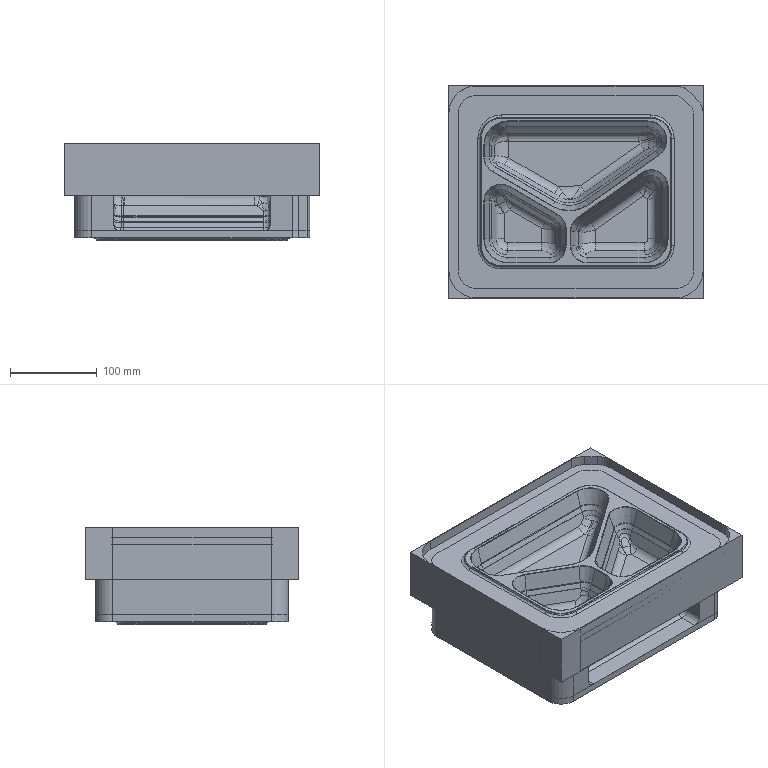NC program | NX | posted with a generic post | part box 295.651 x 246.652 x 112.895 mm
Lines 13478 to 14241 of 299251:
(D2 , TOOL : R2)
N26954 M6
N26956 G53
N26958 G17 G0 G90 X-86.496 Y-88.929 S8000 M3 M8
N26960 G43 Z210.5 H0
N26962 Z54.5
N26964 G94 G1 Z48.888 F4500.
N26966 X-87.187 Y-88.92
N26968 X-87.382
N26970 G2 X-98.418 Y-86.151 R27.034
N26972 G1 X-98.754 Y-85.978 Z48.89
N26974 G2 X-102.06 Y-83.979 R26.069
N26976 G1 X-102.237 Y-83.851 Z48.895
N26978 X-102.421 Y-83.72 Z48.89
N26980 X-102.553 Y-83.622 Z48.894
N26982 X-102.748 Y-83.475 Z48.889
N26984 X-102.871 Y-83.382
N26986 X-103.444 Y-82.929 Z48.89
N26988 X-104.018 Y-82.455 Z48.893
N26990 X-104.148 Y-82.347 Z48.889
N26992 X-104.541 Y-81.998
N26994 X-104.619 Y-81.926 Z48.894
N26996 X-104.763 Y-81.792 Z48.893
N26998 X-105.276 Y-81.305 Z48.889
N27000 X-105.517 Y-81.067 Z48.89
N27002 X-105.627 Y-80.959 Z48.889
N27004 X-106.21 Y-80.354
N27006 X-106.286 Y-80.267
N27008 X-106.349 Y-80.199 Z48.894
N27010 X-106.554 Y-79.97 Z48.89
N27012 X-106.597 Y-79.921 Z48.889
N27014 X-106.793 Y-79.703 Z48.893
N27016 X-106.906 Y-79.578 Z48.889
N27018 G2 X-113.43 Y-61.924 R26.893
N27020 G1 X-113.428 Y61.977 Z48.888
N27022 X-113.411 Y63.015 Z48.889
N27024 G2 X-110.361 Y74.49 R27.082
N27026 G1 X-109.922 Y75.288 Z48.892
N27028 X-109.816 Y75.475 Z48.889
N27030 X-109.67 Y75.733
N27032 X-109.497 Y76.012 Z48.89
N27034 X-109.187 Y76.512 Z48.889
N27036 X-108.966 Y76.853
N27038 X-108.872 Y76.993 Z48.893
N27040 X-108.729 Y77.205 Z48.889
N27042 X-108.632 Y77.35
N27044 X-108.234 Y77.897
N27046 X-108.162 Y77.996 Z48.893
N27048 X-107.984 Y78.24 Z48.889
N27050 X-107.94 Y78.297
N27052 X-107.442 Y78.934
N27054 X-106.904 Y79.579
N27056 X-106.863 Y79.627
N27058 X-106.778 Y79.723 Z48.893
N27060 X-106.553 Y79.974 Z48.89
N27062 X-106.448 Y80.092 Z48.896
N27064 X-106.243 Y80.319 Z48.889
N27066 X-105.865 Y80.712
N27068 X-105.783 Y80.798 Z48.895
N27070 X-105.461 Y81.127 Z48.89
N27072 X-105.222 Y81.356 Z48.889
N27074 X-105.173 Y81.403
N27076 X-105.086 Y81.488 Z48.895
N27078 X-104.861 Y81.703 Z48.889
N27080 X-104.827 Y81.736
N27082 X-104.231 Y82.271 Z48.893
N27084 X-104.136 Y82.356 Z48.889
N27086 G2 X-98.947 Y85.877 R26.524
N27088 G1 X-98.797 Y85.955 Z48.894
N27090 X-98.601 Y86.055 Z48.89
N27092 G2 X-87.533 Y88.91 R26.952
N27094 G1 X-87.187 Y88.917 Z48.888
N27096 X-86.153 Y88.933 Z48.887
N27098 X86.44
N27100 X87.132 Y88.922 Z48.888
N27102 X87.472 Y88.909 Z48.889
N27104 G2 X98.548 Y86.084 R26.934
N27106 G1 X98.774 Y85.97 Z48.893
N27108 X98.895 Y85.908 Z48.889
N27110 X98.997 Y85.857
N27112 X99.24 Y85.726 Z48.89
N27114 X99.446 Y85.614 Z48.894
N27116 X99.586 Y85.538 Z48.889
N27118 X99.635 Y85.511
N27120 X100.24 Y85.165
N27122 X100.279 Y85.139
N27124 X100.971 Y84.711
N27126 X101.18 Y84.578 Z48.895
N27128 X101.426 Y84.417 Z48.889
N27130 X101.856 Y84.127
N27132 X102.008 Y84.016
N27134 X102.697 Y83.516
N27136 X103.25 Y83.088
N27138 X103.826 Y82.614 Z48.893
N27140 X104.082 Y82.402 Z48.889
N27142 X104.337 Y82.177 Z48.895
N27144 X104.429 Y82.095 Z48.889
N27146 X104.482 Y82.05
N27148 X104.565 Y81.975 Z48.894
N27150 X104.709 Y81.844 Z48.893
N27152 X104.773 Y81.785 Z48.889
N27154 G2 X106.239 Y80.319 R36.235
N27156 G1 X106.299 Y80.254 Z48.894
N27158 X106.429 Y80.109
N27160 X106.502 Y80.027 Z48.89
N27162 X106.55 Y79.974 Z48.889
N27164 X106.632 Y79.883 Z48.895
N27166 X106.859 Y79.631 Z48.889
N27168 X107.542 Y78.809
N27170 X108.028 Y78.178 Z48.893
N27172 X108.486 Y77.551 Z48.889
N27174 X108.578 Y77.422
N27176 X108.73 Y77.205
N27178 X108.962 Y76.861
N27180 X109.061 Y76.707 Z48.891
N27182 X109.615 Y75.824 Z48.889
N27184 X110.01 Y75.128
N27186 X110.077 Y75.01 Z48.894
N27188 X110.204 Y74.782 Z48.889
N27190 G2 X113.376 Y63.707 R27.02
N27192 G1 X113.422 Y62.669 Z48.888
N27194 X113.431 Y61.977
N27196 X113.43 Y-61.924
N27198 X113.411 Y-62.963 Z48.889
N27200 G2 X109.844 Y-75.422 R26.888
N27202 G1 X109.723 Y-75.633 Z48.894
N27204 X109.645 Y-75.768 Z48.889
N27206 G2 X107.481 Y-78.883 R25.98
N27208 G1 X106.979 Y-79.487 Z48.894
N27210 X106.904 Y-79.575 Z48.889
N27212 X106.85 Y-79.637
N27214 X106.783 Y-79.715 Z48.894
N27216 X106.603 Y-79.92 Z48.889
N27218 G2 X104.083 Y-82.398 R26.21
N27220 G1 X103.859 Y-82.586 Z48.896
N27222 X103.734 Y-82.69 Z48.89
N27224 X103.476 Y-82.905 Z48.893
N27226 X103.391 Y-82.975 Z48.889
N27228 X103.317 Y-83.034
N27230 X102.7 Y-83.516
N27232 X102.495 Y-83.664 Z48.895
N27234 X102.408 Y-83.726 Z48.89
N27236 X102.354 Y-83.766 Z48.889
N27238 X102.101 Y-83.948 Z48.893
N27240 X102.008 Y-84.015 Z48.889
N27242 G2 X87.385 Y-88.92 R26.931
N27244 G1 X86.141 Y-88.929 Z48.888
N27246 X-86.496
N27248 Y-88.649 Z48.944
N27250 X-87.224 Y-88.639 Z48.938
N27252 X-87.315 Y-88.638 Z48.932
N27254 X-88.225 Y-88.591 Z48.929
N27256 X-88.468 Y-88.574
N27258 X-88.564 Y-88.567 Z48.93
N27260 X-89.263 Y-88.506 Z48.941
N27262 X-89.823 Y-88.442 Z48.948
N27264 X-89.955 Y-88.424 Z48.945
N27266 X-90.128 Y-88.401 Z48.95
N27268 X-90.3 Y-88.375 Z48.945
N27270 X-90.429 Y-88.356 Z48.948
N27272 X-90.646 Y-88.323 Z48.942
N27274 X-90.704 Y-88.315 Z48.943
N27276 X-90.792 Y-88.301 Z48.936
N27278 X-90.992 Y-88.266 Z48.931
N27280 X-91.21 Y-88.228 Z48.93
N27282 X-91.61 Y-88.154 Z48.947
N27284 X-91.684 Y-88.138 Z48.944
N27286 X-91.9 Y-88.098 Z48.951
N27288 X-92.03 Y-88.069 Z48.944
N27290 X-92.185 Y-88.037 Z48.951
N27292 X-92.376 Y-87.993 Z48.942
N27294 X-92.443 Y-87.979 Z48.944
N27296 X-92.529 Y-87.958 Z48.936
N27298 X-92.722 Y-87.911 Z48.931
N27300 X-92.842 Y-87.881
N27302 X-93.299 Y-87.767 Z48.951
N27304 X-93.413 Y-87.733 Z48.944
N27306 X-93.571 Y-87.693 Z48.953
N27308 X-94.122 Y-87.535 Z48.929
N27310 X-94.376 Y-87.461 Z48.949
N27312 X-94.451 Y-87.434 Z48.943
N27314 X-94.64 Y-87.379 Z48.955
N27316 X-94.797 Y-87.326 Z48.942
N27318 X-95.198 Y-87.189 Z48.929
N27320 X-95.672 Y-87.027 Z48.956
N27322 X-95.834 Y-86.963 Z48.941
N27324 X-96.18 Y-86.825 Z48.93
N27326 X-96.355 Y-86.758 Z48.939
N27328 X-96.526 Y-86.69 Z48.943
N27330 X-96.666 Y-86.637 Z48.955
N27332 X-96.872 Y-86.548 Z48.936
N27334 X-96.922 Y-86.526
N27336 X-96.987 Y-86.497 Z48.932
N27338 X-97.151 Y-86.43 Z48.948
N27340 X-97.218 Y-86.398 Z48.941
N27342 X-97.282 Y-86.369 Z48.936
N27344 X-97.51 Y-86.27 Z48.934
N27346 X-97.564 Y-86.245 Z48.933
N27348 X-97.762 Y-86.151 Z48.929
N27350 X-98.101 Y-85.996 Z48.958
N27352 X-98.256 Y-85.917 Z48.94
N27354 X-98.368 Y-85.861
N27356 X-98.474 Y-85.805 Z48.933
N27358 X-98.56 Y-85.764 Z48.943
N27360 X-98.601 Y-85.74 Z48.938
N27362 X-98.791 Y-85.649 Z48.958
N27364 X-98.947 Y-85.563 Z48.941
N27366 X-99.034 Y-85.519 Z48.944
N27368 X-99.147 Y-85.459 Z48.934
N27370 X-99.293 Y-85.378 Z48.939
N27372 X-99.467 Y-85.287 Z48.958
N27374 X-99.639 Y-85.184 Z48.937
N27376 X-99.655 Y-85.175 Z48.938
N27378 X-99.702 Y-85.148
N27380 X-99.761 Y-85.113 Z48.933
N27382 X-99.83 Y-85.074 Z48.937
N27384 X-99.867 Y-85.054 Z48.942
N27386 X-99.985 Y-84.985 Z48.941
N27388 X-100.186 Y-84.867 Z48.943
N27390 X-100.347 Y-84.767 Z48.929
N27392 X-100.677 Y-84.566 Z48.94
N27394 X-100.902 Y-84.42 Z48.93
N27396 X-101.023 Y-84.345 Z48.938
N27398 X-101.045 Y-84.329 Z48.936
N27400 X-101.241 Y-84.202 Z48.93
N27402 X-101.714 Y-83.88 Z48.939
N27404 X-101.925 Y-83.728 Z48.929
N27406 X-102.06 Y-83.632 Z48.939
N27408 X-102.09 Y-83.609 Z48.936
N27410 X-102.287 Y-83.469 Z48.939
N27412 X-102.401 Y-83.382 Z48.93
N27414 X-102.42 Y-83.368
N27416 X-102.752 Y-83.118 Z48.937
N27418 X-102.774 Y-83.101 Z48.938
N27420 X-102.856 Y-83.036 Z48.931
N27422 X-102.969 Y-82.948 Z48.933
N27424 X-103.098 Y-82.848 Z48.939
N27426 X-103.203 Y-82.766 Z48.946
N27428 X-103.292 Y-82.69 Z48.937
N27430 X-103.444 Y-82.567 Z48.939
N27432 X-104.136 Y-81.981 Z48.93
N27434 X-104.294 Y-81.84 Z48.928
N27436 X-104.495 Y-81.655 Z48.93
N27438 X-105.173 Y-81.011 Z48.934
N27440 X-105.614 Y-80.566 Z48.931
N27442 X-105.902 Y-80.267
N27444 X-106.557 Y-79.544 Z48.932
N27446 X-107.119 Y-78.883 Z48.939
N27448 X-107.468 Y-78.444 Z48.93
N27450 X-107.665 Y-78.191 Z48.936
N27452 X-107.976 Y-77.773 Z48.931
N27454 X-108.308 Y-77.315 Z48.928
N27456 X-108.423 Y-77.153 Z48.939
N27458 X-108.7 Y-76.738 Z48.931
N27460 X-108.865 Y-76.489 Z48.937
N27462 X-108.884 Y-76.46 Z48.939
N27464 X-108.978 Y-76.314 Z48.934
N27466 X-109.103 Y-76.114 Z48.94
N27468 X-109.192 Y-75.982 Z48.958
N27470 X-109.315 Y-75.768 Z48.931
N27472 X-109.324 Y-75.754 Z48.93
N27474 X-109.601 Y-75.285 Z48.941
N27476 X-109.67 Y-75.16 Z48.932
N27478 X-109.692 Y-75.122 Z48.935
N27480 X-109.718 Y-75.076 Z48.934
N27482 X-109.829 Y-74.889 Z48.958
N27484 X-109.911 Y-74.73 Z48.941
N27486 X-110.015 Y-74.532 Z48.932
N27488 X-110.036 Y-74.495 Z48.934
N27490 X-110.053 Y-74.461
N27492 X-110.095 Y-74.384 Z48.94
N27494 X-110.189 Y-74.212 Z48.958
N27496 X-110.274 Y-74.038 Z48.94
N27498 X-110.306 Y-73.982 Z48.946
N27500 X-110.361 Y-73.865 Z48.933
N27502 X-110.446 Y-73.692 Z48.939
N27504 X-110.534 Y-73.519 Z48.959
N27506 X-110.612 Y-73.346 Z48.942
N27508 X-110.771 Y-72.999 Z48.93
N27510 X-110.889 Y-72.736 Z48.937
N27512 X-110.926 Y-72.653 Z48.941
N27514 X-110.967 Y-72.567 Z48.95
N27516 X-111.053 Y-72.357 Z48.93
N27518 X-111.22 Y-71.95 Z48.931
N27520 X-111.353 Y-71.615 Z48.936
N27522 X-111.367 Y-71.583 Z48.939
N27524 X-111.399 Y-71.496 Z48.931
N27526 X-111.486 Y-71.269 Z48.94
N27528 X-111.558 Y-71.082 Z48.956
N27530 X-111.61 Y-70.923 Z48.944
N27532 X-111.666 Y-70.764 Z48.938
N27534 X-111.73 Y-70.577 Z48.93
N27536 X-111.745 Y-70.536 Z48.929
N27538 X-111.808 Y-70.356 Z48.938
N27540 X-111.848 Y-70.231 Z48.941
N27542 X-111.908 Y-70.048 Z48.954
N27544 X-112.029 Y-69.638 Z48.934
N27546 X-112.122 Y-69.319 Z48.933
N27548 X-112.219 Y-68.975 Z48.95
N27550 X-112.252 Y-68.846 Z48.944
N27552 X-112.292 Y-68.702 Z48.954
N27554 X-112.437 Y-68.11 Z48.93
N27556 X-112.558 Y-67.584 Z48.948
N27558 X-112.675 Y-66.984 Z48.932
N27560 X-112.717 Y-66.77 Z48.94
N27562 X-112.728 Y-66.715 Z48.942
N27564 X-112.782 Y-66.381 Z48.929
N27566 X-112.833 Y-66.078 Z48.933
N27568 X-112.863 Y-65.893 Z48.936
N27570 X-112.887 Y-65.731 Z48.943
N27572 X-112.915 Y-65.518 Z48.947
N27574 X-112.931 Y-65.385 Z48.944
N27576 X-112.954 Y-65.211 Z48.949
N27578 X-112.974 Y-65.039 Z48.945
N27580 X-112.991 Y-64.901 Z48.949
N27582 X-113.052 Y-64.271 Z48.943
N27584 X-113.099 Y-63.626 Z48.936
N27586 X-113.114 Y-63.309 Z48.934
N27588 X-113.129 Y-62.963 Z48.927
N27590 X-113.148 Y-61.884 Z48.934
N27592 Y62.015
N27594 X-113.128 Y63.006 Z48.927
N27596 X-113.092 Y63.707 Z48.937
N27598 X-113.04 Y64.399 Z48.943
N27600 X-112.986 Y64.949 Z48.949
N27602 X-112.969 Y65.092 Z48.945
N27604 X-112.95 Y65.259 Z48.949
N27606 X-112.871 Y65.847 Z48.944
N27608 X-112.782 Y66.376 Z48.93
N27610 X-112.722 Y66.762 Z48.943
N27612 X-112.71 Y66.822 Z48.94
N27614 X-112.668 Y67.054 Z48.948
N27616 X-112.644 Y67.168 Z48.945
N27618 X-112.61 Y67.342 Z48.953
N27620 X-112.571 Y67.514 Z48.944
N27622 X-112.548 Y67.626 Z48.947
N27624 X-112.498 Y67.86 Z48.937
N27626 X-112.467 Y67.983 Z48.932
N27628 X-112.364 Y68.407 Z48.938
N27630 X-112.329 Y68.552 Z48.945
N27632 X-112.282 Y68.744 Z48.955
N27634 X-112.239 Y68.899 Z48.943
N27636 X-112.209 Y69.017 Z48.948
N27638 X-112.091 Y69.429 Z48.931
N27640 X-112.042 Y69.591 Z48.932
N27642 X-112.022 Y69.66 Z48.933
N27644 X-111.895 Y70.087 Z48.953
N27646 X-111.83 Y70.283 Z48.939
N27648 X-111.781 Y70.428 Z48.933
N27650 X-111.745 Y70.531 Z48.931
N27652 X-111.634 Y70.864 Z48.952
N27654 X-111.592 Y70.975 Z48.944
N27656 X-111.544 Y71.12 Z48.955
N27658 X-111.467 Y71.321 Z48.937
N27660 X-111.443 Y71.386 Z48.938
N27662 X-111.399 Y71.494 Z48.932
N27664 X-111.352 Y71.621 Z48.943
N27666 X-111.331 Y71.667 Z48.939
N27668 X-111.256 Y71.871 Z48.955
N27670 X-111.196 Y72.013 Z48.943
N27672 X-111.164 Y72.095 Z48.948
N27674 X-111.053 Y72.359 Z48.929
N27676 X-110.952 Y72.605 Z48.952
N27678 X-110.904 Y72.706 Z48.941
N27680 X-110.846 Y72.845 Z48.953
N27682 X-110.749 Y73.052 Z48.934
N27684 X-110.729 Y73.092
N27686 X-110.707 Y73.138 Z48.931
N27688 X-110.61 Y73.349 Z48.947
N27690 X-110.585 Y73.398 Z48.944
N27692 X-110.516 Y73.552 Z48.958
N27694 X-110.418 Y73.744 Z48.937
N27696 X-110.415 Y73.751
N27698 X-110.393 Y73.797
N27700 X-110.361 Y73.862 Z48.932
N27702 X-110.29 Y74.018 Z48.949
N27704 X-110.249 Y74.09 Z48.94
N27706 X-110.173 Y74.248 Z48.956
N27708 X-110.015 Y74.534 Z48.929
N27710 X-109.883 Y74.782 Z48.941
N27712 X-109.711 Y75.087 Z48.929
N27714 X-109.688 Y75.128 Z48.93
N27716 X-109.687 Z48.929
N27718 X-109.588 Y75.31 Z48.942
N27720 X-109.493 Y75.474 Z48.94
N27722 X-109.402 Y75.631 Z48.942
N27724 X-109.324 Y75.756 Z48.933
N27726 X-109.284 Y75.82 Z48.935
N27728 X-109.172 Y76.014 Z48.959
N27730 X-109.071 Y76.167 Z48.938
N27732 X-108.955 Y76.351 Z48.93
N27734 X-108.853 Y76.513 Z48.939
N27736 X-108.827 Y76.55 Z48.936
N27738 X-108.715 Y76.723 Z48.94
N27740 X-108.632 Y76.844 Z48.93
N27742 X-108.622 Y76.859 Z48.931
N27744 X-108.492 Y77.065 Z48.958
N27746 X-108.389 Y77.205 Z48.938
N27748 X-108.25 Y77.396 Z48.931
N27750 X-108.139 Y77.551 Z48.939
N27752 X-108.022 Y77.714 Z48.945
N27754 X-107.94 Y77.822 Z48.935
N27756 X-107.886 Y77.897 Z48.937
N27758 X-107.731 Y78.106 Z48.929
N27760 X-107.355 Y78.589 Z48.938
N27762 X-107.329 Y78.624 Z48.941
N27764 X-107.293 Y78.669
N27766 X-107.248 Y78.724 Z48.935
N27768 X-107.075 Y78.935 Z48.938
N27770 X-107.015 Y79.01 Z48.948
N27772 X-106.984 Y79.048
N27774 X-106.903 Y79.142 Z48.936
N27776 X-106.786 Y79.281 Z48.937
N27778 X-106.642 Y79.453 Z48.945
N27780 X-106.557 Y79.547 Z48.934
N27782 X-106.486 Y79.627 Z48.936
N27784 X-106.464 Y79.651 Z48.934
N27786 X-106.331 Y79.804 Z48.95
N27788 X-106.211 Y79.933 Z48.933
N27790 X-106.173 Y79.974 Z48.931
N27792 X-105.865 Y80.305 Z48.93
N27794 X-105.32 Y80.867 Z48.928
N27796 X-104.761 Y81.407 Z48.929
N27798 X-104.481 Y81.667 Z48.931
N27800 X-104.44 Y81.704 Z48.932
N27802 X-104.232 Y81.896 Z48.948
N27804 X-104.136 Y81.978 Z48.936
N27806 X-104.055 Y82.05 Z48.934
N27808 X-103.961 Y82.136 Z48.945
N27810 X-103.79 Y82.279 Z48.937
N27812 X-103.65 Y82.396 Z48.936
N27814 X-103.556 Y82.478 Z48.948
N27816 X-103.519 Y82.509
N27818 X-103.444 Y82.569 Z48.938
N27820 X-103.232 Y82.742 Z48.935
N27822 X-103.098 Y82.848 Z48.932
N27824 X-102.621 Y83.22 Z48.929
N27826 X-102.406 Y83.38 Z48.937
N27828 X-102.387 Y83.395 Z48.94
N27830 X-102.331 Y83.434 Z48.935
N27832 X-102.223 Y83.516 Z48.945
N27834 X-102.06 Y83.632 Z48.939
N27836 X-101.939 Y83.72 Z48.943
N27838 X-101.851 Y83.781 Z48.934
N27840 X-101.791 Y83.824 Z48.941
N27842 X-101.745 Y83.857
N27844 X-101.714 Y83.879 Z48.938
N27846 X-101.573 Y83.985 Z48.958
N27848 X-101.368 Y84.116 Z48.931
N27850 X-101.352 Y84.127 Z48.93
N27852 X-101.232 Y84.208 Z48.94
N27854 X-101.061 Y84.318 Z48.937
N27856 X-101.023 Y84.343 Z48.94
N27858 X-100.91 Y84.416 Z48.942
N27860 X-100.817 Y84.473 Z48.934
N27862 X-100.751 Y84.516 Z48.94
N27864 X-100.703 Y84.546
N27866 X-100.677 Y84.563 Z48.939
N27868 X-100.523 Y84.665 Z48.959
N27870 X-100.331 Y84.778 Z48.936
N27872 X-100.263 Y84.819 Z48.933
N27874 X-100.14 Y84.896 Z48.942
N27876 X-100.073 Y84.938 Z48.949
N27878 X-99.985 Y84.987 Z48.94
N27880 X-99.82 Y85.082 Z48.942
N27882 X-99.639 Y85.182 Z48.928
N27884 X-99.496 Y85.266 Z48.941
N27886 X-99.293 Y85.377
N27888 X-99.041 Y85.511 Z48.933
N27890 X-98.994 Y85.536 Z48.937
N27892 X-98.655 Y85.711 Z48.936
N27894 X-98.601 Y85.738 Z48.933
N27896 X-98.371 Y85.857 Z48.932
N27898 X-98.256 Y85.917 Z48.936
N27900 X-98.067 Y86.014 Z48.957
N27902 X-97.91 Y86.085 Z48.942
N27904 X-97.789 Y86.143 Z48.941
N27906 X-97.744 Y86.162 Z48.936
N27908 X-97.649 Y86.203 Z48.931
N27910 X-97.602 Y86.225 Z48.934
N27912 X-97.565 Y86.241
N27914 X-97.355 Y86.34 Z48.954
N27916 X-97.218 Y86.398 Z48.941
N27918 X-97.116 Y86.447 Z48.952
N27920 X-96.865 Y86.549 Z48.929
N27922 X-96.346 Y86.764 Z48.935
N27924 X-96.009 Y86.895 Z48.931
N27926 X-95.834 Y86.965 Z48.937
N27928 X-95.633 Y87.04 Z48.954
N27930 X-95.489 Y87.087 Z48.944
N27932 X-95.04 Y87.242 Z48.931
N27934 X-94.797 Y87.327 Z48.939
N27936 X-94.6 Y87.391 Z48.953
N27938 X-94.451 Y87.434 Z48.944
N27940 X-94.336 Y87.473 Z48.952
N27942 X-93.938 Y87.588 Z48.931
N27944 X-93.531 Y87.704 Z48.949
N27946 X-93.413 Y87.735 Z48.943
N27948 X-93.259 Y87.779 Z48.954
N27950 X-92.722 Y87.909 Z48.932
N27952 X-92.62 Y87.934 Z48.931
N27954 X-92.378 Y87.994 Z48.937
N27956 X-92.142 Y88.046 Z48.947
N27958 X-92.03 Y88.069 Z48.944
N27960 X-91.858 Y88.108 Z48.953
N27962 X-91.684 Y88.142 Z48.945
N27964 X-91.57 Y88.166 Z48.947
N27966 X-91.338 Y88.208 Z48.94
N27968 X-91.278 Y88.22 Z48.943
N27970 X-90.894 Y88.28 Z48.93
N27972 X-90.646 Y88.32 Z48.933
N27974 X-90.447 Y88.353 Z48.937
N27976 X-90.365 Y88.368 Z48.944
N27978 X-89.776 Y88.447 Z48.949
N27980 X-89.609 Y88.466 Z48.945
N27982 X-89.466 Y88.483 Z48.949
N27984 X-88.837 Y88.546 Z48.943
N27986 X-88.193 Y88.593 Z48.937
N27988 X-87.533 Y88.627 Z48.927
N27990 X-86.445 Y88.651 Z48.933
N27992 X86.493
N27994 X87.161 Y88.639 Z48.929
N27996 X87.481 Y88.627 Z48.928
N27998 X87.816 Y88.615 Z48.933
N28000 X88.519 Y88.573 Z48.938
N28002 X89.21 Y88.51 Z48.945
N28004 X89.418 Y88.488 Z48.949
N28006 X89.556 Y88.471 Z48.945
N28008 X89.728 Y88.452 Z48.949
N28010 X89.902 Y88.429 Z48.944
N28012 X90.33 Y88.373 Z48.945
N28014 X90.587 Y88.333 Z48.937
N28016 X90.594 Y88.331 Z48.933
N28018 X90.94 Y88.272 Z48.931
N28020 X91.231 Y88.225 Z48.942
N28022 X91.286 Y88.214 Z48.94
N28024 X91.503 Y88.171 Z48.933
N28026 X92.1 Y88.056 Z48.948
N28028 X92.422 Y87.983 Z48.936
N28030 X92.616 Y87.934 Z48.93
N28032 X92.669 Y87.921 Z48.931
N28034 X93.217 Y87.789 Z48.954
N28036 X93.361 Y87.749 Z48.943
N28038 X93.49 Y87.716 Z48.949
N28040 X93.945 Y87.588 Z48.931
N28042 X94.399 Y87.451 Z48.944
N28044 X94.561 Y87.404 Z48.954
N28046 X94.745 Y87.343 Z48.941
N28048 X95.09 Y87.224 Z48.93
N28050 X95.275 Y87.161 Z48.939
N28052 X95.436 Y87.106 Z48.944
N28054 X95.594 Y87.053 Z48.956
N28056 X95.893 Y86.94 Z48.934
N28058 X95.923 Y86.928
N28060 X96.004 Y86.895 Z48.93
N28062 X96.128 Y86.848 Z48.936
N28064 X96.346 Y86.767 Z48.954
N28066 X96.474 Y86.713 Z48.942
N28068 X96.581 Y86.672 Z48.95
N28070 X96.866 Y86.549 Z48.93
N28072 X97.079 Y86.463 Z48.95
N28074 X97.166 Y86.421 Z48.941
N28076 X97.481 Y86.282 Z48.931
N28078 X97.512 Y86.268 Z48.93
N28080 X97.857 Y86.108 Z48.942
N28082 X98.031 Y86.031 Z48.958
N28084 X98.29 Y85.899 Z48.934
N28086 X98.318 Y85.884
N28088 X98.371 Y85.857 Z48.931
N28090 X98.53 Y85.779 Z48.941
N28092 X98.549 Y85.768 Z48.94
N28094 X98.723 Y85.685 Z48.958
N28096 X98.895 Y85.593 Z48.939
N28098 X98.916 Y85.582 Z48.94
N28100 X99.077 Y85.493 Z48.932
N28102 X99.241 Y85.406 Z48.941
N28104 X99.4 Y85.324 Z48.958
N28106 X99.672 Y85.165 Z48.928
N28108 X99.933 Y85.017 Z48.94
N28110 X100.116 Y84.91 Z48.943
N28112 X100.261 Y84.819 Z48.931
N28114 X100.279 Y84.808
N28116 X100.492 Y84.686 Z48.958
N28118 X100.624 Y84.598 Z48.94
N28120 X100.787 Y84.493 Z48.929
N28122 X100.819 Y84.473 Z48.928
N28124 X100.97 Y84.378 Z48.939
N28126 X101.126 Y84.282 Z48.958
N28128 X101.351 Y84.127 Z48.931
N28130 X101.662 Y83.917 Z48.939
N28132 X101.825 Y83.8 Z48.928
N28134 X101.852 Y83.781
N28136 X102.008 Y83.67 Z48.939
N28138 X102.418 Y83.37 Z48.93
N28140 X102.757 Y83.114 Z48.937
N28142 X102.79 Y83.088 Z48.934
N28144 X103.046 Y82.891 Z48.938
N28146 X103.106 Y82.845 Z48.945
N28148 X103.148 Y82.811
N28150 X103.228 Y82.742 Z48.936
N28152 X103.563 Y82.468 Z48.944
N28154 X103.646 Y82.396 Z48.935
N28156 X104.107 Y82.003 Z48.93
N28158 X104.292 Y81.841 Z48.928
N28160 X104.44 Y81.707 Z48.93
N28162 X104.813 Y81.358 Z48.931
N28164 X105.479 Y80.705 Z48.935
N28166 X106.161 Y79.985 Z48.93
N28168 X106.504 Y79.603 Z48.931
N28170 X106.659 Y79.436 Z48.958
N28172 X106.785 Y79.281 Z48.936
N28174 X106.85 Y79.204 Z48.934
N28176 X106.93 Y79.112 Z48.943
N28178 X107.305 Y78.653 Z48.928
N28180 X107.542 Y78.348 Z48.931
N28182 X107.607 Y78.266 Z48.939
N28184 X107.624 Y78.243 Z48.937
N28186 X107.878 Y77.907 Z48.93
N28188 X107.888 Y77.894
N28190 X108.038 Y77.701 Z48.959
N28192 X108.14 Y77.551 Z48.938
N28194 X108.234 Y77.42 Z48.933
N28196 X108.266 Y77.376 Z48.935
N28198 X108.315 Y77.309 Z48.941
N28200 X108.602 Y76.891 Z48.93
N28202 X108.624 Y76.859 Z48.934
N28204 X108.748 Y76.681 Z48.959
N28206 X108.851 Y76.513 Z48.938
N28208 X108.926 Y76.395 Z48.932
N28210 X108.957 Y76.346 Z48.934
N28212 X109. Y76.279 Z48.94
N28214 X109.285 Y75.821 Z48.93
N28216 X109.414 Y75.617 Z48.957
N28218 X109.492 Y75.474 Z48.94
N28220 X109.56 Y75.359 Z48.941
N28222 X109.617 Y75.253 Z48.93
N28224 X109.688 Y75.128 Z48.937
N28226 X109.791 Y74.956 Z48.959
N28228 X109.882 Y74.782 Z48.94
N28230 X109.963 Y74.634 Z48.934
N28232 X110.024 Y74.523 Z48.944
N28234 X110.05 Y74.473
N28236 X110.068 Y74.436 Z48.942
N28238 X110.191 Y74.199 Z48.941
N28240 X110.245 Y74.09 Z48.933
N28242 X110.309 Y73.967 Z48.931
N28244 X110.423 Y73.744 Z48.94
N28246 X110.503 Y73.591 Z48.958
N28248 X110.591 Y73.398 Z48.939
N28250 X110.655 Y73.26 Z48.929
N28252 X110.751 Y73.052 Z48.94
N28254 X110.831 Y72.882 Z48.956
N28256 X110.903 Y72.706 Z48.941
N28258 X111.024 Y72.426 Z48.931
N28260 X111.142 Y72.155 Z48.955
N28262 X111.195 Y72.013 Z48.943
N28264 X111.347 Y71.622 Z48.931
N28266 X111.413 Y71.455 Z48.94
N28268 X111.444 Y71.38 Z48.945
N28270 X111.465 Y71.321 Z48.942
N28272 X111.53 Y71.158 Z48.957
N28274 X111.693 Y70.684 Z48.929
N28276 X111.829 Y70.283 Z48.942
N28278 X111.883 Y70.127 Z48.955
N28280 X111.939 Y69.937 Z48.943
N28282 X111.953 Y69.894 Z48.945
N28284 X112.044 Y69.591 Z48.929
N28286 X112.106 Y69.379 Z48.938
N28288 X112.129 Y69.298 Z48.944
N28290 X112.143 Y69.245 Z48.942
N28292 X112.196 Y69.057 Z48.953
N28294 X112.236 Y68.899 Z48.944
N28296 X112.27 Y68.784 Z48.951
N28298 X112.384 Y68.322 Z48.931
N28300 X112.412 Y68.206 Z48.932
N28302 X112.459 Y68.01 Z48.937
N28304 X112.48 Y67.928 Z48.944
N28306 X112.495 Y67.86 Z48.942
N28308 X112.539 Y67.669 Z48.951
N28310 X112.57 Y67.514 Z48.945
N28312 X112.6 Y67.384 Z48.952
N28314 X112.642 Y67.168 Z48.944
N28316 X112.658 Y67.096 Z48.946
N28318 X112.73 Y66.683 Z48.93
N28320 X112.801 Y66.272 Z48.936
N28322 X112.816 Y66.186 Z48.944
N28324 X112.824 Y66.13 Z48.943
N28326 X112.858 Y65.912 Z48.948
N28328 X112.876 Y65.784 Z48.945
N28330 X112.901 Y65.608 Z48.951
N28332 X112.921 Y65.438 Z48.946
N28334 X112.939 Y65.301 Z48.949
N28336 X113.012 Y64.682 Z48.943
N28338 X113.092 Y63.707 Z48.929
N28340 X113.123 Y63.109 Z48.934
N28342 X113.127 Y63.015 Z48.933
N28344 X113.136 Y62.788 Z48.932
N28346 X113.141 Y62.683 Z48.938
N28348 X113.152 Y61.706 Z48.943
N28350 X113.151 Y-61.999
N28352 X113.139 Y-62.639 Z48.938
N28354 X113.136 Y-62.737 Z48.933
N28356 X113.114 Y-63.309 Z48.934
N28358 X113.076 Y-63.916 Z48.929
N28360 X113.049 Y-64.32 Z48.936
N28362 X113.046 Y-64.347 Z48.935
N28364 X112.987 Y-64.95 Z48.944
N28366 X112.933 Y-65.385
N28368 X112.911 Y-65.566 Z48.949
N28370 X112.887 Y-65.731 Z48.945
N28372 X112.868 Y-65.869 Z48.948
N28374 X112.778 Y-66.414 Z48.936
N28376 X112.716 Y-66.77 Z48.93
N28378 X112.667 Y-67.024
N28380 X112.647 Y-67.128
N28382 X112.549 Y-67.627 Z48.952
N28384 X112.507 Y-67.808 Z48.943
N28386 X112.488 Y-67.896 Z48.946
N28388 X112.428 Y-68.147 Z48.935
N28390 X112.426 Y-68.154 Z48.932
N28392 X112.355 Y-68.442 Z48.937
N28394 X112.282 Y-68.744 Z48.949
N28396 X112.253 Y-68.846 Z48.943
N28398 X112.21 Y-69.018 Z48.953
N28400 X112.16 Y-69.192 Z48.942
N28402 X112.14 Y-69.266 Z48.945
N28404 X112.038 Y-69.609 Z48.93
N28406 X111.895 Y-70.087 Z48.954
N28408 X111.846 Y-70.231 Z48.942
N28410 X111.812 Y-70.343 Z48.948
N28412 X111.732 Y-70.574 Z48.933
N28414 X111.73 Y-70.577 Z48.931
N28416 X111.693 Y-70.684
N28418 X111.633 Y-70.864 Z48.947
N28420 X111.61 Y-70.923 Z48.942
N28422 X111.544 Y-71.12 Z48.956
N28424 X111.486 Y-71.269 Z48.942
N28426 X111.457 Y-71.35 Z48.947
N28428 X111.353 Y-71.613 Z48.928
N28430 X111.347 Y-71.63
N28432 X111.275 Y-71.817 Z48.939
N28434 X111.218 Y-71.961 Z48.942
N28436 X111.159 Y-72.119 Z48.956
N28438 X111.077 Y-72.307 Z48.939
N28440 X111.07 Y-72.324 Z48.94
N28442 X111.047 Y-72.377
N28444 X111.001 Y-72.48 Z48.933
N28446 X110.951 Y-72.603 Z48.944
N28448 X110.927 Y-72.653 Z48.939
N28450 X110.732 Y-73.095 Z48.929
N28452 X110.613 Y-73.346 Z48.937
N28454 X110.519 Y-73.555 Z48.957
N28456 X110.447 Y-73.692 Z48.941
N28458 X110.379 Y-73.831
N28460 X110.309 Y-73.966 Z48.932
N28462 X110.273 Y-74.038
N28464 X110.123 Y-74.337 Z48.944
N28466 X109.963 Y-74.634 Z48.932
N28468 X109.912 Y-74.73 Z48.937
N28470 X109.811 Y-74.924 Z48.958
N28472 X109.719 Y-75.076 Z48.939
N28474 X109.701 Y-75.11 Z48.942